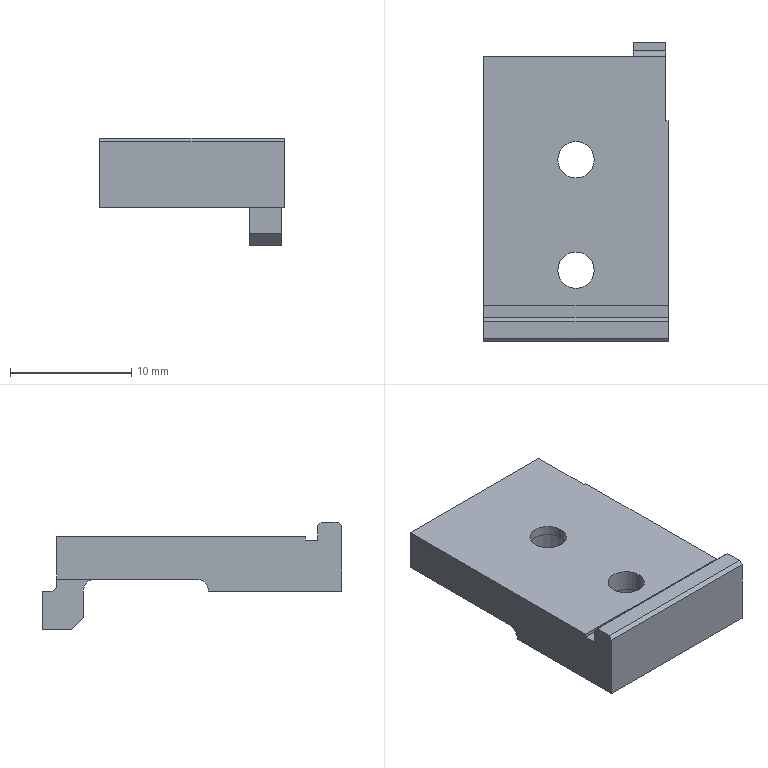Part | NX | 1 solid | 34 faces | box 15.2 x 24.7 x 8.9 mm | volume 1358 mm3 | plane 23 | cylinder 11 | commonest cylinder face diameters 3 x4 5 x4 2 x2 1 x1
STEP:
#1=CARTESIAN_POINT('',(-15.2,-12.7,1.));
#2=VERTEX_POINT('',#1);
#3=CARTESIAN_POINT('',(-15.2,-1.2,1.));
#4=VERTEX_POINT('',#3);
#5=CARTESIAN_POINT('',(-15.2,0.,1.));
#6=DIRECTION('',(0.,1.,0.));
#7=VECTOR('',#6,1000.);
#8=LINE('',#5,#7);
#9=EDGE_CURVE('',#2,#4,#8,.T.);
#10=ORIENTED_EDGE('',*,*,#9,.F.);
#11=CARTESIAN_POINT('',(-15.2,-13.7,0.));
#12=VERTEX_POINT('',#11);
#13=CARTESIAN_POINT('',(-15.2,-12.7,0.));
#14=DIRECTION('',(1.,0.,0.));
#15=DIRECTION('',(0.,-1.,0.));
#16=AXIS2_PLACEMENT_3D('',#13,#14,#15);
#17=CIRCLE('',#16,1.);
#18=EDGE_CURVE('',#2,#12,#17,.T.);
#19=ORIENTED_EDGE('',*,*,#18,.T.);
#20=CARTESIAN_POINT('',(-15.2,-24.7,0.));
#21=VERTEX_POINT('',#20);
#22=CARTESIAN_POINT('',(-15.2,0.,0.));
#23=DIRECTION('',(0.,1.,0.));
#24=VECTOR('',#23,1000.);
#25=LINE('',#22,#24);
#26=EDGE_CURVE('',#21,#12,#25,.T.);
#27=ORIENTED_EDGE('',*,*,#26,.F.);
#28=CARTESIAN_POINT('',(-15.2,-24.7,5.4));
#29=VERTEX_POINT('',#28);
#30=CARTESIAN_POINT('',(-15.2,-24.7,0.));
#31=DIRECTION('',(0.,0.,-1.));
#32=VECTOR('',#31,1000.);
#33=LINE('',#30,#32);
#34=EDGE_CURVE('',#29,#21,#33,.T.);
#35=ORIENTED_EDGE('',*,*,#34,.F.);
#36=CARTESIAN_POINT('',(-15.2,-24.4,5.7));
#37=VERTEX_POINT('',#36);
#38=CARTESIAN_POINT('',(-15.2,0.,30.1));
#39=DIRECTION('',(0.,0.7071,0.7071));
#40=VECTOR('',#39,1000.);
#41=LINE('',#38,#40);
#42=EDGE_CURVE('',#29,#37,#41,.T.);
#43=ORIENTED_EDGE('',*,*,#42,.T.);
#44=CARTESIAN_POINT('',(-15.2,-23.,5.7));
#45=VERTEX_POINT('',#44);
#46=CARTESIAN_POINT('',(-15.2,0.,5.7));
#47=DIRECTION('',(0.,1.,0.));
#48=VECTOR('',#47,1000.);
#49=LINE('',#46,#48);
#50=EDGE_CURVE('',#37,#45,#49,.T.);
#51=ORIENTED_EDGE('',*,*,#50,.T.);
#52=CARTESIAN_POINT('',(-15.2,-22.7,5.4));
#53=VERTEX_POINT('',#52);
#54=CARTESIAN_POINT('',(-15.2,0.,-17.3));
#55=DIRECTION('',(0.,-0.7071,0.7071));
#56=VECTOR('',#55,1000.);
#57=LINE('',#54,#56);
#58=EDGE_CURVE('',#53,#45,#57,.T.);
#59=ORIENTED_EDGE('',*,*,#58,.F.);
#60=CARTESIAN_POINT('',(-15.2,-22.7,4.2));
#61=VERTEX_POINT('',#60);
#62=CARTESIAN_POINT('',(-15.2,-22.7,0.));
#63=DIRECTION('',(0.,0.,-1.));
#64=VECTOR('',#63,1000.);
#65=LINE('',#62,#64);
#66=EDGE_CURVE('',#53,#61,#65,.T.);
#67=ORIENTED_EDGE('',*,*,#66,.T.);
#68=CARTESIAN_POINT('',(-15.2,-21.7,4.2));
#69=VERTEX_POINT('',#68);
#70=CARTESIAN_POINT('',(-15.2,0.,4.2));
#71=DIRECTION('',(0.,-1.,0.));
#72=VECTOR('',#71,1000.);
#73=LINE('',#70,#72);
#74=EDGE_CURVE('',#69,#61,#73,.T.);
#75=ORIENTED_EDGE('',*,*,#74,.F.);
#76=CARTESIAN_POINT('',(-15.2,-21.7,4.5));
#77=VERTEX_POINT('',#76);
#78=CARTESIAN_POINT('',(-15.2,-21.7,0.));
#79=DIRECTION('',(0.,0.,-1.));
#80=VECTOR('',#79,1000.);
#81=LINE('',#78,#80);
#82=EDGE_CURVE('',#77,#69,#81,.T.);
#83=ORIENTED_EDGE('',*,*,#82,.F.);
#84=CARTESIAN_POINT('',(-15.2,-1.2,4.5));
#85=VERTEX_POINT('',#84);
#86=CARTESIAN_POINT('',(-15.2,0.,4.5));
#87=DIRECTION('',(0.,-1.,0.));
#88=VECTOR('',#87,1000.);
#89=LINE('',#86,#88);
#90=EDGE_CURVE('',#85,#77,#89,.T.);
#91=ORIENTED_EDGE('',*,*,#90,.F.);
#92=CARTESIAN_POINT('',(-15.2,-1.2,0.));
#93=DIRECTION('',(0.,0.,1.));
#94=VECTOR('',#93,1000.);
#95=LINE('',#92,#94);
#96=EDGE_CURVE('',#4,#85,#95,.T.);
#97=ORIENTED_EDGE('',*,*,#96,.F.);
#98=EDGE_LOOP('',(#10,#19,#27,#35,#43,#51,#59,#67,#75,#83,#91,#97));
#99=FACE_BOUND('',#98,.T.);
#100=CARTESIAN_POINT('',(-15.2,0.,0.));
#101=DIRECTION('',(1.,0.,0.));
#102=DIRECTION('',(0.,1.,0.));
#103=AXIS2_PLACEMENT_3D('',#100,#101,#102);
#104=PLANE('',#103);
#105=ADVANCED_FACE('',(#99),#104,.F.);
#106=CARTESIAN_POINT('',(0.,-21.7,4.5));
#107=VERTEX_POINT('',#106);
#108=CARTESIAN_POINT('',(0.,-6.5,4.5));
#109=VERTEX_POINT('',#108);
#110=CARTESIAN_POINT('',(0.,0.,4.5));
#111=DIRECTION('',(0.,1.,0.));
#112=VECTOR('',#111,1000.);
#113=LINE('',#110,#112);
#114=EDGE_CURVE('',#107,#109,#113,.T.);
#115=ORIENTED_EDGE('',*,*,#114,.F.);
#116=CARTESIAN_POINT('',(0.,-21.7,4.2));
#117=VERTEX_POINT('',#116);
#118=CARTESIAN_POINT('',(0.,-21.7,0.));
#119=DIRECTION('',(0.,0.,1.));
#120=VECTOR('',#119,1000.);
#121=LINE('',#118,#120);
#122=EDGE_CURVE('',#117,#107,#121,.T.);
#123=ORIENTED_EDGE('',*,*,#122,.F.);
#124=CARTESIAN_POINT('',(0.,-22.7,4.2));
#125=VERTEX_POINT('',#124);
#126=CARTESIAN_POINT('',(0.,0.,4.2));
#127=DIRECTION('',(0.,1.,0.));
#128=VECTOR('',#127,1000.);
#129=LINE('',#126,#128);
#130=EDGE_CURVE('',#125,#117,#129,.T.);
#131=ORIENTED_EDGE('',*,*,#130,.F.);
#132=CARTESIAN_POINT('',(0.,-22.7,5.4));
#133=VERTEX_POINT('',#132);
#134=CARTESIAN_POINT('',(0.,-22.7,0.));
#135=DIRECTION('',(0.,0.,1.));
#136=VECTOR('',#135,1000.);
#137=LINE('',#134,#136);
#138=EDGE_CURVE('',#125,#133,#137,.T.);
#139=ORIENTED_EDGE('',*,*,#138,.T.);
#140=CARTESIAN_POINT('',(0.,-23.,5.7));
#141=VERTEX_POINT('',#140);
#142=CARTESIAN_POINT('',(0.,0.,-17.3));
#143=DIRECTION('',(0.,0.7071,-0.7071));
#144=VECTOR('',#143,1000.);
#145=LINE('',#142,#144);
#146=EDGE_CURVE('',#141,#133,#145,.T.);
#147=ORIENTED_EDGE('',*,*,#146,.F.);
#148=CARTESIAN_POINT('',(0.,-24.4,5.7));
#149=VERTEX_POINT('',#148);
#150=CARTESIAN_POINT('',(0.,0.,5.7));
#151=DIRECTION('',(0.,-1.,0.));
#152=VECTOR('',#151,1000.);
#153=LINE('',#150,#152);
#154=EDGE_CURVE('',#141,#149,#153,.T.);
#155=ORIENTED_EDGE('',*,*,#154,.T.);
#156=CARTESIAN_POINT('',(0.,-24.7,5.4));
#157=VERTEX_POINT('',#156);
#158=CARTESIAN_POINT('',(0.,0.,30.1));
#159=DIRECTION('',(0.,-0.7071,-0.7071));
#160=VECTOR('',#159,1000.);
#161=LINE('',#158,#160);
#162=EDGE_CURVE('',#149,#157,#161,.T.);
#163=ORIENTED_EDGE('',*,*,#162,.T.);
#164=CARTESIAN_POINT('',(0.,-24.7,0.));
#165=VERTEX_POINT('',#164);
#166=CARTESIAN_POINT('',(0.,-24.7,0.));
#167=DIRECTION('',(0.,0.,1.));
#168=VECTOR('',#167,1000.);
#169=LINE('',#166,#168);
#170=EDGE_CURVE('',#165,#157,#169,.T.);
#171=ORIENTED_EDGE('',*,*,#170,.F.);
#172=CARTESIAN_POINT('',(0.,-13.7,0.));
#173=VERTEX_POINT('',#172);
#174=CARTESIAN_POINT('',(0.,0.,0.));
#175=DIRECTION('',(0.,-1.,0.));
#176=VECTOR('',#175,1000.);
#177=LINE('',#174,#176);
#178=EDGE_CURVE('',#173,#165,#177,.T.);
#179=ORIENTED_EDGE('',*,*,#178,.F.);
#180=CARTESIAN_POINT('',(0.,-12.7,1.));
#181=VERTEX_POINT('',#180);
#182=CARTESIAN_POINT('',(0.,-12.7,0.));
#183=DIRECTION('',(1.,0.,0.));
#184=DIRECTION('',(0.,-1.,0.));
#185=AXIS2_PLACEMENT_3D('',#182,#183,#184);
#186=CIRCLE('',#185,1.);
#187=EDGE_CURVE('',#181,#173,#186,.T.);
#188=ORIENTED_EDGE('',*,*,#187,.F.);
#189=CARTESIAN_POINT('',(0.,-6.5,1.));
#190=VERTEX_POINT('',#189);
#191=CARTESIAN_POINT('',(0.,0.,1.));
#192=DIRECTION('',(0.,-1.,0.));
#193=VECTOR('',#192,1000.);
#194=LINE('',#191,#193);
#195=EDGE_CURVE('',#190,#181,#194,.T.);
#196=ORIENTED_EDGE('',*,*,#195,.F.);
#197=CARTESIAN_POINT('',(0.,-6.5,0.));
#198=DIRECTION('',(0.,0.,-1.));
#199=VECTOR('',#198,1000.);
#200=LINE('',#197,#199);
#201=EDGE_CURVE('',#109,#190,#200,.T.);
#202=ORIENTED_EDGE('',*,*,#201,.F.);
#203=EDGE_LOOP('',(#115,#123,#131,#139,#147,#155,#163,#171,#179,#188,#196,#202));
#204=FACE_BOUND('',#203,.T.);
#205=CARTESIAN_POINT('',(0.,-24.7,0.));
#206=DIRECTION('',(-1.,0.,0.));
#207=DIRECTION('',(0.,0.,1.));
#208=AXIS2_PLACEMENT_3D('',#205,#206,#207);
#209=PLANE('',#208);
#210=ADVANCED_FACE('',(#204),#209,.F.);
#211=CARTESIAN_POINT('',(-5.1,-18.8,2.7));
#212=VERTEX_POINT('',#211);
#213=CARTESIAN_POINT('',(-10.1,-18.8,2.7));
#214=VERTEX_POINT('',#213);
#215=CARTESIAN_POINT('',(-7.6,-18.8,2.7));
#216=DIRECTION('',(0.,0.,-1.));
#217=DIRECTION('',(-1.,0.,0.));
#218=AXIS2_PLACEMENT_3D('',#215,#216,#217);
#219=CIRCLE('',#218,2.5);
#220=EDGE_CURVE('',#212,#214,#219,.T.);
#221=ORIENTED_EDGE('',*,*,#220,.T.);
#222=CARTESIAN_POINT('',(-7.6,-18.8,2.7));
#223=DIRECTION('',(0.,0.,-1.));
#224=DIRECTION('',(-1.,0.,0.));
#225=AXIS2_PLACEMENT_3D('',#222,#223,#224);
#226=CIRCLE('',#225,2.5);
#227=EDGE_CURVE('',#214,#212,#226,.T.);
#228=ORIENTED_EDGE('',*,*,#227,.T.);
#229=EDGE_LOOP('',(#221,#228));
#230=FACE_BOUND('',#229,.T.);
#231=CARTESIAN_POINT('',(-6.1,-18.8,2.7));
#232=VERTEX_POINT('',#231);
#233=CARTESIAN_POINT('',(-9.1,-18.8,2.7));
#234=VERTEX_POINT('',#233);
#235=CARTESIAN_POINT('',(-7.6,-18.8,2.7));
#236=DIRECTION('',(0.,0.,-1.));
#237=DIRECTION('',(-1.,0.,0.));
#238=AXIS2_PLACEMENT_3D('',#235,#236,#237);
#239=CIRCLE('',#238,1.5);
#240=EDGE_CURVE('',#232,#234,#239,.T.);
#241=ORIENTED_EDGE('',*,*,#240,.F.);
#242=CARTESIAN_POINT('',(-7.6,-18.8,2.7));
#243=DIRECTION('',(0.,0.,-1.));
#244=DIRECTION('',(-1.,0.,0.));
#245=AXIS2_PLACEMENT_3D('',#242,#243,#244);
#246=CIRCLE('',#245,1.5);
#247=EDGE_CURVE('',#234,#232,#246,.T.);
#248=ORIENTED_EDGE('',*,*,#247,.F.);
#249=EDGE_LOOP('',(#241,#248));
#250=FACE_BOUND('',#249,.T.);
#251=CARTESIAN_POINT('',(-11.486,-5.592,2.7));
#252=DIRECTION('',(0.,0.,-1.));
#253=DIRECTION('',(0.,-1.,0.));
#254=AXIS2_PLACEMENT_3D('',#251,#252,#253);
#255=PLANE('',#254);
#256=ADVANCED_FACE('',(#230,#250),#255,.T.);
#257=CARTESIAN_POINT('',(-0.2,-4.4,1.));
#258=VERTEX_POINT('',#257);
#259=CARTESIAN_POINT('',(-2.9,-4.4,1.));
#260=VERTEX_POINT('',#259);
#261=CARTESIAN_POINT('',(0.,-4.4,1.));
#262=DIRECTION('',(-1.,0.,0.));
#263=VECTOR('',#262,1000.);
#264=LINE('',#261,#263);
#265=EDGE_CURVE('',#258,#260,#264,.T.);
#266=ORIENTED_EDGE('',*,*,#265,.F.);
#267=CARTESIAN_POINT('',(-0.2,-6.5,1.));
#268=VERTEX_POINT('',#267);
#269=CARTESIAN_POINT('',(-0.2,0.,1.));
#270=DIRECTION('',(0.,1.,0.));
#271=VECTOR('',#270,1000.);
#272=LINE('',#269,#271);
#273=EDGE_CURVE('',#268,#258,#272,.T.);
#274=ORIENTED_EDGE('',*,*,#273,.F.);
#275=CARTESIAN_POINT('',(0.,-6.5,1.));
#276=DIRECTION('',(-1.,0.,0.));
#277=VECTOR('',#276,1000.);
#278=LINE('',#275,#277);
#279=EDGE_CURVE('',#190,#268,#278,.T.);
#280=ORIENTED_EDGE('',*,*,#279,.F.);
#281=ORIENTED_EDGE('',*,*,#195,.T.);
#282=CARTESIAN_POINT('',(0.,-12.7,1.));
#283=DIRECTION('',(1.,0.,0.));
#284=VECTOR('',#283,1000.);
#285=LINE('',#282,#284);
#286=EDGE_CURVE('',#2,#181,#285,.T.);
#287=ORIENTED_EDGE('',*,*,#286,.F.);
#288=ORIENTED_EDGE('',*,*,#9,.T.);
#289=CARTESIAN_POINT('',(-2.9,-1.2,1.));
#290=VERTEX_POINT('',#289);
#291=CARTESIAN_POINT('',(0.,-1.2,1.));
#292=DIRECTION('',(-1.,0.,0.));
#293=VECTOR('',#292,1000.);
#294=LINE('',#291,#293);
#295=EDGE_CURVE('',#290,#4,#294,.T.);
#296=ORIENTED_EDGE('',*,*,#295,.F.);
#297=CARTESIAN_POINT('',(-2.9,0.,1.));
#298=DIRECTION('',(0.,1.,0.));
#299=VECTOR('',#298,1000.);
#300=LINE('',#297,#299);
#301=EDGE_CURVE('',#260,#290,#300,.T.);
#302=ORIENTED_EDGE('',*,*,#301,.F.);
#303=EDGE_LOOP('',(#266,#274,#280,#281,#287,#288,#296,#302));
#304=FACE_BOUND('',#303,.T.);
#305=CARTESIAN_POINT('',(-10.1,-9.7,1.));
#306=VERTEX_POINT('',#305);
#307=CARTESIAN_POINT('',(-5.1,-9.7,1.));
#308=VERTEX_POINT('',#307);
#309=CARTESIAN_POINT('',(-7.6,-9.7,1.));
#310=DIRECTION('',(0.,0.,-1.));
#311=DIRECTION('',(-1.,0.,0.));
#312=AXIS2_PLACEMENT_3D('',#309,#310,#311);
#313=CIRCLE('',#312,2.5);
#314=EDGE_CURVE('',#306,#308,#313,.T.);
#315=ORIENTED_EDGE('',*,*,#314,.F.);
#316=CARTESIAN_POINT('',(-7.6,-9.7,1.));
#317=DIRECTION('',(0.,0.,-1.));
#318=DIRECTION('',(-1.,0.,0.));
#319=AXIS2_PLACEMENT_3D('',#316,#317,#318);
#320=CIRCLE('',#319,2.5);
#321=EDGE_CURVE('',#308,#306,#320,.T.);
#322=ORIENTED_EDGE('',*,*,#321,.F.);
#323=EDGE_LOOP('',(#315,#322));
#324=FACE_BOUND('',#323,.T.);
#325=CARTESIAN_POINT('',(-11.724,-4.43,1.));
#326=DIRECTION('',(0.,0.,-1.));
#327=DIRECTION('',(0.,-1.,0.));
#328=AXIS2_PLACEMENT_3D('',#325,#326,#327);
#329=PLANE('',#328);
#330=ADVANCED_FACE('',(#304,#324),#329,.T.);
#331=CARTESIAN_POINT('',(-0.2,-3.4,-2.2));
#332=VERTEX_POINT('',#331);
#333=CARTESIAN_POINT('',(-0.2,-3.4,0.));
#334=VERTEX_POINT('',#333);
#335=CARTESIAN_POINT('',(-0.2,-3.4,0.));
#336=DIRECTION('',(0.,0.,1.));
#337=VECTOR('',#336,1000.);
#338=LINE('',#335,#337);
#339=EDGE_CURVE('',#332,#334,#338,.T.);
#340=ORIENTED_EDGE('',*,*,#339,.F.);
#341=CARTESIAN_POINT('',(-0.2,-2.4,-3.2));
#342=VERTEX_POINT('',#341);
#343=CARTESIAN_POINT('',(-0.2,-5.6,0.));
#344=DIRECTION('',(0.,0.7071,-0.7071));
#345=VECTOR('',#344,1000.);
#346=LINE('',#343,#345);
#347=EDGE_CURVE('',#332,#342,#346,.T.);
#348=ORIENTED_EDGE('',*,*,#347,.T.);
#349=CARTESIAN_POINT('',(-0.2,0.,-3.2));
#350=VERTEX_POINT('',#349);
#351=CARTESIAN_POINT('',(-0.2,0.,-3.2));
#352=DIRECTION('',(0.,-1.,0.));
#353=VECTOR('',#352,1000.);
#354=LINE('',#351,#353);
#355=EDGE_CURVE('',#350,#342,#354,.T.);
#356=ORIENTED_EDGE('',*,*,#355,.F.);
#357=CARTESIAN_POINT('',(-0.2,0.,0.));
#358=VERTEX_POINT('',#357);
#359=CARTESIAN_POINT('',(-0.2,0.,0.));
#360=DIRECTION('',(0.,0.,-1.));
#361=VECTOR('',#360,1000.);
#362=LINE('',#359,#361);
#363=EDGE_CURVE('',#358,#350,#362,.T.);
#364=ORIENTED_EDGE('',*,*,#363,.F.);
#365=CARTESIAN_POINT('',(-0.2,-0.7,0.));
#366=VERTEX_POINT('',#365);
#367=CARTESIAN_POINT('',(-0.2,0.,0.));
#368=DIRECTION('',(0.,-1.,0.));
#369=VECTOR('',#368,1000.);
#370=LINE('',#367,#369);
#371=EDGE_CURVE('',#358,#366,#370,.T.);
#372=ORIENTED_EDGE('',*,*,#371,.T.);
#373=CARTESIAN_POINT('',(-0.2,-1.2,0.5));
#374=VERTEX_POINT('',#373);
#375=CARTESIAN_POINT('',(-0.2,-0.7,0.5));
#376=DIRECTION('',(-1.,0.,0.));
#377=DIRECTION('',(0.,1.,0.));
#378=AXIS2_PLACEMENT_3D('',#375,#376,#377);
#379=CIRCLE('',#378,0.5);
#380=EDGE_CURVE('',#366,#374,#379,.T.);
#381=ORIENTED_EDGE('',*,*,#380,.T.);
#382=CARTESIAN_POINT('',(-0.2,-1.2,4.5));
#383=VERTEX_POINT('',#382);
#384=CARTESIAN_POINT('',(-0.2,-1.2,0.));
#385=DIRECTION('',(0.,0.,1.));
#386=VECTOR('',#385,1000.);
#387=LINE('',#384,#386);
#388=EDGE_CURVE('',#374,#383,#387,.T.);
#389=ORIENTED_EDGE('',*,*,#388,.T.);
#390=CARTESIAN_POINT('',(-0.2,-6.5,4.5));
#391=VERTEX_POINT('',#390);
#392=CARTESIAN_POINT('',(-0.2,0.,4.5));
#393=DIRECTION('',(0.,-1.,0.));
#394=VECTOR('',#393,1000.);
#395=LINE('',#392,#394);
#396=EDGE_CURVE('',#383,#391,#395,.T.);
#397=ORIENTED_EDGE('',*,*,#396,.T.);
#398=CARTESIAN_POINT('',(-0.2,-6.5,0.));
#399=DIRECTION('',(0.,0.,1.));
#400=VECTOR('',#399,1000.);
#401=LINE('',#398,#400);
#402=EDGE_CURVE('',#268,#391,#401,.T.);
#403=ORIENTED_EDGE('',*,*,#402,.F.);
#404=ORIENTED_EDGE('',*,*,#273,.T.);
#405=CARTESIAN_POINT('',(-0.2,-4.4,0.));
#406=DIRECTION('',(-1.,0.,0.));
#407=DIRECTION('',(0.,1.,0.));
#408=AXIS2_PLACEMENT_3D('',#405,#406,#407);
#409=CIRCLE('',#408,1.);
#410=EDGE_CURVE('',#258,#334,#409,.T.);
#411=ORIENTED_EDGE('',*,*,#410,.T.);
#412=EDGE_LOOP('',(#340,#348,#356,#364,#372,#381,#389,#397,#403,#404,#411));
#413=FACE_BOUND('',#412,.T.);
#414=CARTESIAN_POINT('',(-0.2,-6.5,2.));
#415=DIRECTION('',(1.,0.,0.));
#416=DIRECTION('',(0.,1.,0.));
#417=AXIS2_PLACEMENT_3D('',#414,#415,#416);
#418=PLANE('',#417);
#419=ADVANCED_FACE('',(#413),#418,.T.);
#420=ORIENTED_EDGE('',*,*,#82,.T.);
#421=CARTESIAN_POINT('',(0.,-21.7,4.2));
#422=DIRECTION('',(1.,0.,0.));
#423=VECTOR('',#422,1000.);
#424=LINE('',#421,#423);
#425=EDGE_CURVE('',#69,#117,#424,.T.);
#426=ORIENTED_EDGE('',*,*,#425,.T.);
#427=ORIENTED_EDGE('',*,*,#122,.T.);
#428=CARTESIAN_POINT('',(0.,-21.7,4.5));
#429=DIRECTION('',(1.,0.,0.));
#430=VECTOR('',#429,1000.);
#431=LINE('',#428,#430);
#432=EDGE_CURVE('',#77,#107,#431,.T.);
#433=ORIENTED_EDGE('',*,*,#432,.F.);
#434=EDGE_LOOP('',(#420,#426,#427,#433));
#435=FACE_BOUND('',#434,.T.);
#436=CARTESIAN_POINT('',(0.,-21.7,2.));
#437=DIRECTION('',(0.,-1.,0.));
#438=DIRECTION('',(0.,0.,-1.));
#439=AXIS2_PLACEMENT_3D('',#436,#437,#438);
#440=PLANE('',#439);
#441=ADVANCED_FACE('',(#435),#440,.T.);
#442=CARTESIAN_POINT('',(-2.9,-3.4,-2.2));
#443=VERTEX_POINT('',#442);
#444=CARTESIAN_POINT('',(-2.9,-3.4,0.));
#445=VERTEX_POINT('',#444);
#446=CARTESIAN_POINT('',(-2.9,-3.4,0.));
#447=DIRECTION('',(0.,0.,1.));
#448=VECTOR('',#447,1000.);
#449=LINE('',#446,#448);
#450=EDGE_CURVE('',#443,#445,#449,.T.);
#451=ORIENTED_EDGE('',*,*,#450,.T.);
#452=CARTESIAN_POINT('',(-2.9,-4.4,0.));
#453=DIRECTION('',(-1.,0.,0.));
#454=DIRECTION('',(0.,1.,0.));
#455=AXIS2_PLACEMENT_3D('',#452,#453,#454);
#456=CIRCLE('',#455,1.);
#457=EDGE_CURVE('',#260,#445,#456,.T.);
#458=ORIENTED_EDGE('',*,*,#457,.F.);
#459=ORIENTED_EDGE('',*,*,#301,.T.);
#460=CARTESIAN_POINT('',(-2.9,-1.2,0.5));
#461=VERTEX_POINT('',#460);
#462=CARTESIAN_POINT('',(-2.9,-1.2,0.));
#463=DIRECTION('',(0.,0.,1.));
#464=VECTOR('',#463,1000.);
#465=LINE('',#462,#464);
#466=EDGE_CURVE('',#461,#290,#465,.T.);
#467=ORIENTED_EDGE('',*,*,#466,.F.);
#468=CARTESIAN_POINT('',(-2.9,-0.7,0.));
#469=VERTEX_POINT('',#468);
#470=CARTESIAN_POINT('',(-2.9,-0.7,0.5));
#471=DIRECTION('',(-1.,0.,0.));
#472=DIRECTION('',(0.,1.,0.));
#473=AXIS2_PLACEMENT_3D('',#470,#471,#472);
#474=CIRCLE('',#473,0.5);
#475=EDGE_CURVE('',#469,#461,#474,.T.);
#476=ORIENTED_EDGE('',*,*,#475,.F.);
#477=CARTESIAN_POINT('',(-2.9,0.,0.));
#478=VERTEX_POINT('',#477);
#479=CARTESIAN_POINT('',(-2.9,0.,0.));
#480=DIRECTION('',(0.,-1.,0.));
#481=VECTOR('',#480,1000.);
#482=LINE('',#479,#481);
#483=EDGE_CURVE('',#478,#469,#482,.T.);
#484=ORIENTED_EDGE('',*,*,#483,.F.);
#485=CARTESIAN_POINT('',(-2.9,0.,-3.2));
#486=VERTEX_POINT('',#485);
#487=CARTESIAN_POINT('',(-2.9,0.,0.));
#488=DIRECTION('',(0.,0.,-1.));
#489=VECTOR('',#488,1000.);
#490=LINE('',#487,#489);
#491=EDGE_CURVE('',#478,#486,#490,.T.);
#492=ORIENTED_EDGE('',*,*,#491,.T.);
#493=CARTESIAN_POINT('',(-2.9,-2.4,-3.2));
#494=VERTEX_POINT('',#493);
#495=CARTESIAN_POINT('',(-2.9,0.,-3.2));
#496=DIRECTION('',(0.,1.,0.));
#497=VECTOR('',#496,1000.);
#498=LINE('',#495,#497);
#499=EDGE_CURVE('',#494,#486,#498,.T.);
#500=ORIENTED_EDGE('',*,*,#499,.F.);
#501=CARTESIAN_POINT('',(-2.9,-5.6,0.));
#502=DIRECTION('',(0.,0.7071,-0.7071));
#503=VECTOR('',#502,1000.);
#504=LINE('',#501,#503);
#505=EDGE_CURVE('',#443,#494,#504,.T.);
#506=ORIENTED_EDGE('',*,*,#505,.F.);
#507=EDGE_LOOP('',(#451,#458,#459,#467,#476,#484,#492,#500,#506));
#508=FACE_BOUND('',#507,.T.);
#509=CARTESIAN_POINT('',(-2.9,-1.2,0.));
#510=DIRECTION('',(1.,0.,0.));
#511=DIRECTION('',(0.,1.,0.));
#512=AXIS2_PLACEMENT_3D('',#509,#510,#511);
#513=PLANE('',#512);
#514=ADVANCED_FACE('',(#508),#513,.F.);
#515=ORIENTED_EDGE('',*,*,#279,.T.);
#516=ORIENTED_EDGE('',*,*,#402,.T.);
#517=CARTESIAN_POINT('',(0.,-6.5,4.5));
#518=DIRECTION('',(-1.,0.,0.));
#519=VECTOR('',#518,1000.);
#520=LINE('',#517,#519);
#521=EDGE_CURVE('',#109,#391,#520,.T.);
#522=ORIENTED_EDGE('',*,*,#521,.F.);
#523=ORIENTED_EDGE('',*,*,#201,.T.);
#524=EDGE_LOOP('',(#515,#516,#522,#523));
#525=FACE_BOUND('',#524,.T.);
#526=CARTESIAN_POINT('',(0.,-6.5,2.));
#527=DIRECTION('',(0.,1.,0.));
#528=DIRECTION('',(1.,0.,0.));
#529=AXIS2_PLACEMENT_3D('',#526,#527,#528);
#530=PLANE('',#529);
#531=ADVANCED_FACE('',(#525),#530,.T.);
#532=CARTESIAN_POINT('',(0.,-13.7,0.));
#533=DIRECTION('',(1.,0.,0.));
#534=VECTOR('',#533,1000.);
#535=LINE('',#532,#534);
#536=EDGE_CURVE('',#12,#173,#535,.T.);
#537=ORIENTED_EDGE('',*,*,#536,.T.);
#538=ORIENTED_EDGE('',*,*,#178,.T.);
#539=CARTESIAN_POINT('',(-15.2,-24.7,0.));
#540=DIRECTION('',(1.,0.,0.));
#541=VECTOR('',#540,1000.);
#542=LINE('',#539,#541);
#543=EDGE_CURVE('',#21,#165,#542,.T.);
#544=ORIENTED_EDGE('',*,*,#543,.F.);
#545=ORIENTED_EDGE('',*,*,#26,.T.);
#546=EDGE_LOOP('',(#537,#538,#544,#545));
#547=FACE_BOUND('',#546,.T.);
#548=CARTESIAN_POINT('',(-10.1,-18.8,0.));
#549=VERTEX_POINT('',#548);
#550=CARTESIAN_POINT('',(-5.1,-18.8,0.));
#551=VERTEX_POINT('',#550);
#552=CARTESIAN_POINT('',(-7.6,-18.8,0.));
#553=DIRECTION('',(0.,0.,-1.));
#554=DIRECTION('',(-1.,0.,0.));
#555=AXIS2_PLACEMENT_3D('',#552,#553,#554);
#556=CIRCLE('',#555,2.5);
#557=EDGE_CURVE('',#549,#551,#556,.T.);
#558=ORIENTED_EDGE('',*,*,#557,.F.);
#559=CARTESIAN_POINT('',(-7.6,-18.8,0.));
#560=DIRECTION('',(0.,0.,-1.));
#561=DIRECTION('',(-1.,0.,0.));
#562=AXIS2_PLACEMENT_3D('',#559,#560,#561);
#563=CIRCLE('',#562,2.5);
#564=EDGE_CURVE('',#551,#549,#563,.T.);
#565=ORIENTED_EDGE('',*,*,#564,.F.);
#566=EDGE_LOOP('',(#558,#565));
#567=FACE_BOUND('',#566,.T.);
#568=CARTESIAN_POINT('',(-11.977,-15.053,0.));
#569=DIRECTION('',(0.,0.,-1.));
#570=DIRECTION('',(0.,-1.,0.));
#571=AXIS2_PLACEMENT_3D('',#568,#569,#570);
#572=PLANE('',#571);
#573=ADVANCED_FACE('',(#547,#567),#572,.T.);
#574=ORIENTED_EDGE('',*,*,#371,.F.);
#575=CARTESIAN_POINT('',(0.,0.,0.));
#576=DIRECTION('',(1.,0.,0.));
#577=VECTOR('',#576,1000.);
#578=LINE('',#575,#577);
#579=EDGE_CURVE('',#478,#358,#578,.T.);
#580=ORIENTED_EDGE('',*,*,#579,.F.);
#581=ORIENTED_EDGE('',*,*,#483,.T.);
#582=CARTESIAN_POINT('',(0.,-0.7,0.));
#583=DIRECTION('',(-1.,0.,0.));
#584=VECTOR('',#583,1000.);
#585=LINE('',#582,#584);
#586=EDGE_CURVE('',#366,#469,#585,.T.);
#587=ORIENTED_EDGE('',*,*,#586,.F.);
#588=EDGE_LOOP('',(#574,#580,#581,#587));
#589=FACE_BOUND('',#588,.T.);
#590=CARTESIAN_POINT('',(-15.2,-1.2,0.));
#591=DIRECTION('',(0.,0.,1.));
#592=DIRECTION('',(1.,0.,0.));
#593=AXIS2_PLACEMENT_3D('',#590,#591,#592);
#594=PLANE('',#593);
#595=ADVANCED_FACE('',(#589),#594,.T.);
#596=CARTESIAN_POINT('',(0.,0.,-3.2));
#597=DIRECTION('',(1.,0.,0.));
#598=VECTOR('',#597,1000.);
#599=LINE('',#596,#598);
#600=EDGE_CURVE('',#486,#350,#599,.T.);
#601=ORIENTED_EDGE('',*,*,#600,.F.);
#602=ORIENTED_EDGE('',*,*,#491,.F.);
#603=ORIENTED_EDGE('',*,*,#579,.T.);
#604=ORIENTED_EDGE('',*,*,#363,.T.);
#605=EDGE_LOOP('',(#601,#602,#603,#604));
#606=FACE_BOUND('',#605,.T.);
#607=CARTESIAN_POINT('',(0.,0.,0.));
#608=DIRECTION('',(0.,-1.,0.));
#609=DIRECTION('',(0.,0.,-1.));
#610=AXIS2_PLACEMENT_3D('',#607,#608,#609);
#611=PLANE('',#610);
#612=ADVANCED_FACE('',(#606),#611,.F.);
#613=CARTESIAN_POINT('',(0.,-2.4,-3.2));
#614=DIRECTION('',(1.,0.,0.));
#615=VECTOR('',#614,1000.);
#616=LINE('',#613,#615);
#617=EDGE_CURVE('',#494,#342,#616,.T.);
#618=ORIENTED_EDGE('',*,*,#617,.F.);
#619=ORIENTED_EDGE('',*,*,#499,.T.);
#620=ORIENTED_EDGE('',*,*,#600,.T.);
#621=ORIENTED_EDGE('',*,*,#355,.T.);
#622=EDGE_LOOP('',(#618,#619,#620,#621));
#623=FACE_BOUND('',#622,.T.);
#624=CARTESIAN_POINT('',(0.,0.,-3.2));
#625=DIRECTION('',(0.,0.,1.));
#626=DIRECTION('',(1.,0.,0.));
#627=AXIS2_PLACEMENT_3D('',#624,#625,#626);
#628=PLANE('',#627);
#629=ADVANCED_FACE('',(#623),#628,.F.);
#630=CARTESIAN_POINT('',(0.,-22.7,4.2));
#631=DIRECTION('',(1.,0.,0.));
#632=VECTOR('',#631,1000.);
#633=LINE('',#630,#632);
#634=EDGE_CURVE('',#61,#125,#633,.T.);
#635=ORIENTED_EDGE('',*,*,#634,.T.);
#636=ORIENTED_EDGE('',*,*,#130,.T.);
#637=ORIENTED_EDGE('',*,*,#425,.F.);
#638=ORIENTED_EDGE('',*,*,#74,.T.);
#639=EDGE_LOOP('',(#635,#636,#637,#638));
#640=FACE_BOUND('',#639,.T.);
#641=CARTESIAN_POINT('',(0.,-21.7,4.2));
#642=DIRECTION('',(0.,0.,1.));
#643=DIRECTION('',(1.,0.,0.));
#644=AXIS2_PLACEMENT_3D('',#641,#642,#643);
#645=PLANE('',#644);
#646=ADVANCED_FACE('',(#640),#645,.T.);
#647=ORIENTED_EDGE('',*,*,#450,.F.);
#648=CARTESIAN_POINT('',(0.,-3.4,-2.2));
#649=DIRECTION('',(-1.,0.,0.));
#650=VECTOR('',#649,1000.);
#651=LINE('',#648,#650);
#652=EDGE_CURVE('',#332,#443,#651,.T.);
#653=ORIENTED_EDGE('',*,*,#652,.F.);
#654=ORIENTED_EDGE('',*,*,#339,.T.);
#655=CARTESIAN_POINT('',(0.,-3.4,0.));
#656=DIRECTION('',(-1.,0.,0.));
#657=VECTOR('',#656,1000.);
#658=LINE('',#655,#657);
#659=EDGE_CURVE('',#334,#445,#658,.T.);
#660=ORIENTED_EDGE('',*,*,#659,.T.);
#661=EDGE_LOOP('',(#647,#653,#654,#660));
#662=FACE_BOUND('',#661,.T.);
#663=CARTESIAN_POINT('',(-15.2,-3.4,0.));
#664=DIRECTION('',(0.,1.,0.));
#665=DIRECTION('',(1.,0.,0.));
#666=AXIS2_PLACEMENT_3D('',#663,#664,#665);
#667=PLANE('',#666);
#668=ADVANCED_FACE('',(#662),#667,.F.);
#669=CARTESIAN_POINT('',(0.,-1.2,0.5));
#670=DIRECTION('',(-1.,0.,0.));
#671=VECTOR('',#670,1000.);
#672=LINE('',#669,#671);
#673=EDGE_CURVE('',#374,#461,#672,.T.);
#674=ORIENTED_EDGE('',*,*,#673,.T.);
#675=ORIENTED_EDGE('',*,*,#466,.T.);
#676=ORIENTED_EDGE('',*,*,#295,.T.);
#677=ORIENTED_EDGE('',*,*,#96,.T.);
#678=CARTESIAN_POINT('',(0.,-1.2,4.5));
#679=DIRECTION('',(-1.,0.,0.));
#680=VECTOR('',#679,1000.);
#681=LINE('',#678,#680);
#682=EDGE_CURVE('',#383,#85,#681,.T.);
#683=ORIENTED_EDGE('',*,*,#682,.F.);
#684=ORIENTED_EDGE('',*,*,#388,.F.);
#685=EDGE_LOOP('',(#674,#675,#676,#677,#683,#684));
#686=FACE_BOUND('',#685,.T.);
#687=CARTESIAN_POINT('',(-15.2,-1.2,2.));
#688=DIRECTION('',(0.,1.,0.));
#689=DIRECTION('',(1.,0.,0.));
#690=AXIS2_PLACEMENT_3D('',#687,#688,#689);
#691=PLANE('',#690);
#692=ADVANCED_FACE('',(#686),#691,.T.);
#693=ORIENTED_EDGE('',*,*,#286,.T.);
#694=ORIENTED_EDGE('',*,*,#187,.T.);
#695=ORIENTED_EDGE('',*,*,#536,.F.);
#696=ORIENTED_EDGE('',*,*,#18,.F.);
#697=EDGE_LOOP('',(#693,#694,#695,#696));
#698=FACE_BOUND('',#697,.T.);
#699=CARTESIAN_POINT('',(0.,-12.7,0.));
#700=DIRECTION('',(1.,0.,0.));
#701=DIRECTION('',(0.,-1.,0.));
#702=AXIS2_PLACEMENT_3D('',#699,#700,#701);
#703=CYLINDRICAL_SURFACE('',#702,1.);
#704=ADVANCED_FACE('',(#698),#703,.F.);
#705=CARTESIAN_POINT('',(0.,-23.,5.7));
#706=DIRECTION('',(-1.,0.,0.));
#707=VECTOR('',#706,1000.);
#708=LINE('',#705,#707);
#709=EDGE_CURVE('',#141,#45,#708,.T.);
#710=ORIENTED_EDGE('',*,*,#709,.T.);
#711=ORIENTED_EDGE('',*,*,#50,.F.);
#712=CARTESIAN_POINT('',(0.,-24.4,5.7));
#713=DIRECTION('',(-1.,0.,0.));
#714=VECTOR('',#713,1000.);
#715=LINE('',#712,#714);
#716=EDGE_CURVE('',#149,#37,#715,.T.);
#717=ORIENTED_EDGE('',*,*,#716,.F.);
#718=ORIENTED_EDGE('',*,*,#154,.F.);
#719=EDGE_LOOP('',(#710,#711,#717,#718));
#720=FACE_BOUND('',#719,.T.);
#721=CARTESIAN_POINT('',(0.,-22.7,5.7));
#722=DIRECTION('',(0.,0.,-1.));
#723=DIRECTION('',(0.,-1.,0.));
#724=AXIS2_PLACEMENT_3D('',#721,#722,#723);
#725=PLANE('',#724);
#726=ADVANCED_FACE('',(#720),#725,.F.);
#727=ORIENTED_EDGE('',*,*,#634,.F.);
#728=ORIENTED_EDGE('',*,*,#66,.F.);
#729=CARTESIAN_POINT('',(0.,-22.7,5.4));
#730=DIRECTION('',(1.,0.,0.));
#731=VECTOR('',#730,1000.);
#732=LINE('',#729,#731);
#733=EDGE_CURVE('',#53,#133,#732,.T.);
#734=ORIENTED_EDGE('',*,*,#733,.T.);
#735=ORIENTED_EDGE('',*,*,#138,.F.);
#736=EDGE_LOOP('',(#727,#728,#734,#735));
#737=FACE_BOUND('',#736,.T.);
#738=CARTESIAN_POINT('',(0.,-22.7,2.));
#739=DIRECTION('',(0.,-1.,0.));
#740=DIRECTION('',(0.,0.,-1.));
#741=AXIS2_PLACEMENT_3D('',#738,#739,#740);
#742=PLANE('',#741);
#743=ADVANCED_FACE('',(#737),#742,.F.);
#744=ORIENTED_EDGE('',*,*,#709,.F.);
#745=ORIENTED_EDGE('',*,*,#146,.T.);
#746=ORIENTED_EDGE('',*,*,#733,.F.);
#747=ORIENTED_EDGE('',*,*,#58,.T.);
#748=EDGE_LOOP('',(#744,#745,#746,#747));
#749=FACE_BOUND('',#748,.T.);
#750=CARTESIAN_POINT('',(-7.6,-22.85,5.55));
#751=DIRECTION('',(0.,0.7071,0.7071));
#752=DIRECTION('',(1.,0.,0.));
#753=AXIS2_PLACEMENT_3D('',#750,#751,#752);
#754=PLANE('',#753);
#755=ADVANCED_FACE('',(#749),#754,.T.);
#756=ORIENTED_EDGE('',*,*,#557,.T.);
#757=CARTESIAN_POINT('',(-5.1,-18.8,0.));
#758=DIRECTION('',(0.,0.,-1.));
#759=VECTOR('',#758,1000.);
#760=LINE('',#757,#759);
#761=EDGE_CURVE('',#212,#551,#760,.T.);
#762=ORIENTED_EDGE('',*,*,#761,.F.);
#763=ORIENTED_EDGE('',*,*,#227,.F.);
#764=CARTESIAN_POINT('',(-10.1,-18.8,0.));
#765=DIRECTION('',(0.,0.,-1.));
#766=VECTOR('',#765,1000.);
#767=LINE('',#764,#766);
#768=EDGE_CURVE('',#214,#549,#767,.T.);
#769=ORIENTED_EDGE('',*,*,#768,.T.);
#770=EDGE_LOOP('',(#756,#762,#763,#769));
#771=FACE_BOUND('',#770,.T.);
#772=CARTESIAN_POINT('',(-7.6,-18.8,0.));
#773=DIRECTION('',(0.,0.,-1.));
#774=DIRECTION('',(-1.,0.,0.));
#775=AXIS2_PLACEMENT_3D('',#772,#773,#774);
#776=CYLINDRICAL_SURFACE('',#775,2.5);
#777=ADVANCED_FACE('',(#771),#776,.F.);
#778=ORIENTED_EDGE('',*,*,#314,.T.);
#779=CARTESIAN_POINT('',(-5.1,-9.7,3.7));
#780=VERTEX_POINT('',#779);
#781=CARTESIAN_POINT('',(-5.1,-9.7,0.));
#782=DIRECTION('',(0.,0.,-1.));
#783=VECTOR('',#782,1000.);
#784=LINE('',#781,#783);
#785=EDGE_CURVE('',#780,#308,#784,.T.);
#786=ORIENTED_EDGE('',*,*,#785,.F.);
#787=CARTESIAN_POINT('',(-10.1,-9.7,3.7));
#788=VERTEX_POINT('',#787);
#789=CARTESIAN_POINT('',(-7.6,-9.7,3.7));
#790=DIRECTION('',(0.,0.,-1.));
#791=DIRECTION('',(-1.,0.,0.));
#792=AXIS2_PLACEMENT_3D('',#789,#790,#791);
#793=CIRCLE('',#792,2.5);
#794=EDGE_CURVE('',#788,#780,#793,.T.);
#795=ORIENTED_EDGE('',*,*,#794,.F.);
#796=CARTESIAN_POINT('',(-10.1,-9.7,0.));
#797=DIRECTION('',(0.,0.,-1.));
#798=VECTOR('',#797,1000.);
#799=LINE('',#796,#798);
#800=EDGE_CURVE('',#788,#306,#799,.T.);
#801=ORIENTED_EDGE('',*,*,#800,.T.);
#802=EDGE_LOOP('',(#778,#786,#795,#801));
#803=FACE_BOUND('',#802,.T.);
#804=CARTESIAN_POINT('',(-7.6,-9.7,0.));
#805=DIRECTION('',(0.,0.,-1.));
#806=DIRECTION('',(-1.,0.,0.));
#807=AXIS2_PLACEMENT_3D('',#804,#805,#806);
#808=CYLINDRICAL_SURFACE('',#807,2.5);
#809=ADVANCED_FACE('',(#803),#808,.F.);
#810=CARTESIAN_POINT('',(0.,-24.7,5.4));
#811=DIRECTION('',(1.,0.,0.));
#812=VECTOR('',#811,1000.);
#813=LINE('',#810,#812);
#814=EDGE_CURVE('',#29,#157,#813,.T.);
#815=ORIENTED_EDGE('',*,*,#814,.T.);
#816=ORIENTED_EDGE('',*,*,#162,.F.);
#817=ORIENTED_EDGE('',*,*,#716,.T.);
#818=ORIENTED_EDGE('',*,*,#42,.F.);
#819=EDGE_LOOP('',(#815,#816,#817,#818));
#820=FACE_BOUND('',#819,.T.);
#821=CARTESIAN_POINT('',(-7.6,-24.55,5.55));
#822=DIRECTION('',(0.,0.7071,-0.7071));
#823=DIRECTION('',(-1.,0.,0.));
#824=AXIS2_PLACEMENT_3D('',#821,#822,#823);
#825=PLANE('',#824);
#826=ADVANCED_FACE('',(#820),#825,.F.);
#827=CARTESIAN_POINT('',(-9.1,-9.7,4.5));
#828=VERTEX_POINT('',#827);
#829=CARTESIAN_POINT('',(-6.1,-9.7,4.5));
#830=VERTEX_POINT('',#829);
#831=CARTESIAN_POINT('',(-7.6,-9.7,4.5));
#832=DIRECTION('',(0.,0.,-1.));
#833=DIRECTION('',(-1.,0.,0.));
#834=AXIS2_PLACEMENT_3D('',#831,#832,#833);
#835=CIRCLE('',#834,1.5);
#836=EDGE_CURVE('',#828,#830,#835,.T.);
#837=ORIENTED_EDGE('',*,*,#836,.F.);
#838=CARTESIAN_POINT('',(-9.1,-9.7,3.7));
#839=VERTEX_POINT('',#838);
#840=CARTESIAN_POINT('',(-9.1,-9.7,5.45));
#841=DIRECTION('',(0.,0.,-1.));
#842=VECTOR('',#841,1000.);
#843=LINE('',#840,#842);
#844=EDGE_CURVE('',#839,#828,#843,.F.);
#845=ORIENTED_EDGE('',*,*,#844,.F.);
#846=CARTESIAN_POINT('',(-6.1,-9.7,3.7));
#847=VERTEX_POINT('',#846);
#848=CARTESIAN_POINT('',(-7.6,-9.7,3.7));
#849=DIRECTION('',(0.,0.,-1.));
#850=DIRECTION('',(-1.,0.,0.));
#851=AXIS2_PLACEMENT_3D('',#848,#849,#850);
#852=CIRCLE('',#851,1.5);
#853=EDGE_CURVE('',#839,#847,#852,.T.);
#854=ORIENTED_EDGE('',*,*,#853,.T.);
#855=CARTESIAN_POINT('',(-6.1,-9.7,5.45));
#856=DIRECTION('',(0.,0.,-1.));
#857=VECTOR('',#856,1000.);
#858=LINE('',#855,#857);
#859=EDGE_CURVE('',#847,#830,#858,.F.);
#860=ORIENTED_EDGE('',*,*,#859,.T.);
#861=EDGE_LOOP('',(#837,#845,#854,#860));
#862=FACE_BOUND('',#861,.T.);
#863=CARTESIAN_POINT('',(-7.6,-9.7,5.45));
#864=DIRECTION('',(0.,0.,-1.));
#865=DIRECTION('',(-1.,0.,0.));
#866=AXIS2_PLACEMENT_3D('',#863,#864,#865);
#867=CYLINDRICAL_SURFACE('',#866,1.5);
#868=ADVANCED_FACE('',(#862),#867,.F.);
#869=ORIENTED_EDGE('',*,*,#240,.T.);
#870=CARTESIAN_POINT('',(-9.1,-18.8,4.5));
#871=VERTEX_POINT('',#870);
#872=CARTESIAN_POINT('',(-9.1,-18.8,5.45));
#873=DIRECTION('',(0.,0.,-1.));
#874=VECTOR('',#873,1000.);
#875=LINE('',#872,#874);
#876=EDGE_CURVE('',#234,#871,#875,.F.);
#877=ORIENTED_EDGE('',*,*,#876,.T.);
#878=CARTESIAN_POINT('',(-6.1,-18.8,4.5));
#879=VERTEX_POINT('',#878);
#880=CARTESIAN_POINT('',(-7.6,-18.8,4.5));
#881=DIRECTION('',(0.,0.,-1.));
#882=DIRECTION('',(-1.,0.,0.));
#883=AXIS2_PLACEMENT_3D('',#880,#881,#882);
#884=CIRCLE('',#883,1.5);
#885=EDGE_CURVE('',#879,#871,#884,.T.);
#886=ORIENTED_EDGE('',*,*,#885,.F.);
#887=CARTESIAN_POINT('',(-6.1,-18.8,5.45));
#888=DIRECTION('',(0.,0.,-1.));
#889=VECTOR('',#888,1000.);
#890=LINE('',#887,#889);
#891=EDGE_CURVE('',#232,#879,#890,.F.);
#892=ORIENTED_EDGE('',*,*,#891,.F.);
#893=EDGE_LOOP('',(#869,#877,#886,#892));
#894=FACE_BOUND('',#893,.T.);
#895=CARTESIAN_POINT('',(-7.6,-18.8,5.45));
#896=DIRECTION('',(0.,0.,-1.));
#897=DIRECTION('',(-1.,0.,0.));
#898=AXIS2_PLACEMENT_3D('',#895,#896,#897);
#899=CYLINDRICAL_SURFACE('',#898,1.5);
#900=ADVANCED_FACE('',(#894),#899,.F.);
#901=ORIENTED_EDGE('',*,*,#396,.F.);
#902=ORIENTED_EDGE('',*,*,#682,.T.);
#903=ORIENTED_EDGE('',*,*,#90,.T.);
#904=ORIENTED_EDGE('',*,*,#432,.T.);
#905=ORIENTED_EDGE('',*,*,#114,.T.);
#906=ORIENTED_EDGE('',*,*,#521,.T.);
#907=EDGE_LOOP('',(#901,#902,#903,#904,#905,#906));
#908=FACE_BOUND('',#907,.T.);
#909=ORIENTED_EDGE('',*,*,#836,.T.);
#910=CARTESIAN_POINT('',(-7.6,-9.7,4.5));
#911=DIRECTION('',(0.,0.,-1.));
#912=DIRECTION('',(-1.,0.,0.));
#913=AXIS2_PLACEMENT_3D('',#910,#911,#912);
#914=CIRCLE('',#913,1.5);
#915=EDGE_CURVE('',#830,#828,#914,.T.);
#916=ORIENTED_EDGE('',*,*,#915,.T.);
#917=EDGE_LOOP('',(#909,#916));
#918=FACE_BOUND('',#917,.T.);
#919=CARTESIAN_POINT('',(-7.6,-18.8,4.5));
#920=DIRECTION('',(0.,0.,-1.));
#921=DIRECTION('',(-1.,0.,0.));
#922=AXIS2_PLACEMENT_3D('',#919,#920,#921);
#923=CIRCLE('',#922,1.5);
#924=EDGE_CURVE('',#871,#879,#923,.T.);
#925=ORIENTED_EDGE('',*,*,#924,.T.);
#926=ORIENTED_EDGE('',*,*,#885,.T.);
#927=EDGE_LOOP('',(#925,#926));
#928=FACE_BOUND('',#927,.T.);
#929=CARTESIAN_POINT('',(0.,0.,4.5));
#930=DIRECTION('',(0.,0.,1.));
#931=DIRECTION('',(1.,0.,0.));
#932=AXIS2_PLACEMENT_3D('',#929,#930,#931);
#933=PLANE('',#932);
#934=ADVANCED_FACE('',(#908,#918,#928),#933,.T.);
#935=CARTESIAN_POINT('',(-7.6,-9.7,3.7));
#936=DIRECTION('',(0.,0.,-1.));
#937=DIRECTION('',(-1.,0.,0.));
#938=AXIS2_PLACEMENT_3D('',#935,#936,#937);
#939=CIRCLE('',#938,2.5);
#940=EDGE_CURVE('',#780,#788,#939,.T.);
#941=ORIENTED_EDGE('',*,*,#940,.T.);
#942=ORIENTED_EDGE('',*,*,#794,.T.);
#943=EDGE_LOOP('',(#941,#942));
#944=FACE_BOUND('',#943,.T.);
#945=CARTESIAN_POINT('',(-7.6,-9.7,3.7));
#946=DIRECTION('',(0.,0.,-1.));
#947=DIRECTION('',(-1.,0.,0.));
#948=AXIS2_PLACEMENT_3D('',#945,#946,#947);
#949=CIRCLE('',#948,1.5);
#950=EDGE_CURVE('',#847,#839,#949,.T.);
#951=ORIENTED_EDGE('',*,*,#950,.F.);
#952=ORIENTED_EDGE('',*,*,#853,.F.);
#953=EDGE_LOOP('',(#951,#952));
#954=FACE_BOUND('',#953,.T.);
#955=CARTESIAN_POINT('',(-11.486,-5.592,3.7));
#956=DIRECTION('',(0.,0.,-1.));
#957=DIRECTION('',(0.,-1.,0.));
#958=AXIS2_PLACEMENT_3D('',#955,#956,#957);
#959=PLANE('',#958);
#960=ADVANCED_FACE('',(#944,#954),#959,.T.);
#961=ORIENTED_EDGE('',*,*,#673,.F.);
#962=ORIENTED_EDGE('',*,*,#380,.F.);
#963=ORIENTED_EDGE('',*,*,#586,.T.);
#964=ORIENTED_EDGE('',*,*,#475,.T.);
#965=EDGE_LOOP('',(#961,#962,#963,#964));
#966=FACE_BOUND('',#965,.T.);
#967=CARTESIAN_POINT('',(0.,-0.7,0.5));
#968=DIRECTION('',(-1.,0.,0.));
#969=DIRECTION('',(0.,1.,0.));
#970=AXIS2_PLACEMENT_3D('',#967,#968,#969);
#971=CYLINDRICAL_SURFACE('',#970,0.5);
#972=ADVANCED_FACE('',(#966),#971,.F.);
#973=ORIENTED_EDGE('',*,*,#34,.T.);
#974=ORIENTED_EDGE('',*,*,#543,.T.);
#975=ORIENTED_EDGE('',*,*,#170,.T.);
#976=ORIENTED_EDGE('',*,*,#814,.F.);
#977=EDGE_LOOP('',(#973,#974,#975,#976));
#978=FACE_BOUND('',#977,.T.);
#979=CARTESIAN_POINT('',(-15.2,-24.7,1.));
#980=DIRECTION('',(0.,-1.,0.));
#981=DIRECTION('',(0.,0.,-1.));
#982=AXIS2_PLACEMENT_3D('',#979,#980,#981);
#983=PLANE('',#982);
#984=ADVANCED_FACE('',(#978),#983,.T.);
#985=ORIENTED_EDGE('',*,*,#265,.T.);
#986=ORIENTED_EDGE('',*,*,#457,.T.);
#987=ORIENTED_EDGE('',*,*,#659,.F.);
#988=ORIENTED_EDGE('',*,*,#410,.F.);
#989=EDGE_LOOP('',(#985,#986,#987,#988));
#990=FACE_BOUND('',#989,.T.);
#991=CARTESIAN_POINT('',(0.,-4.4,0.));
#992=DIRECTION('',(-1.,0.,0.));
#993=DIRECTION('',(0.,1.,0.));
#994=AXIS2_PLACEMENT_3D('',#991,#992,#993);
#995=CYLINDRICAL_SURFACE('',#994,1.);
#996=ADVANCED_FACE('',(#990),#995,.F.);
#997=ORIENTED_EDGE('',*,*,#617,.T.);
#998=ORIENTED_EDGE('',*,*,#347,.F.);
#999=ORIENTED_EDGE('',*,*,#652,.T.);
#1000=ORIENTED_EDGE('',*,*,#505,.T.);
#1001=EDGE_LOOP('',(#997,#998,#999,#1000));
#1002=FACE_BOUND('',#1001,.T.);
#1003=CARTESIAN_POINT('',(-1.55,-2.9,-2.7));
#1004=DIRECTION('',(0.,-0.7071,-0.7071));
#1005=DIRECTION('',(0.,-0.7071,0.7071));
#1006=AXIS2_PLACEMENT_3D('',#1003,#1004,#1005);
#1007=PLANE('',#1006);
#1008=ADVANCED_FACE('',(#1002),#1007,.T.);
#1009=ORIENTED_EDGE('',*,*,#950,.T.);
#1010=ORIENTED_EDGE('',*,*,#844,.T.);
#1011=ORIENTED_EDGE('',*,*,#915,.F.);
#1012=ORIENTED_EDGE('',*,*,#859,.F.);
#1013=EDGE_LOOP('',(#1009,#1010,#1011,#1012));
#1014=FACE_BOUND('',#1013,.T.);
#1015=CARTESIAN_POINT('',(-7.6,-9.7,5.45));
#1016=DIRECTION('',(0.,0.,-1.));
#1017=DIRECTION('',(-1.,0.,0.));
#1018=AXIS2_PLACEMENT_3D('',#1015,#1016,#1017);
#1019=CYLINDRICAL_SURFACE('',#1018,1.5);
#1020=ADVANCED_FACE('',(#1014),#1019,.F.);
#1021=ORIENTED_EDGE('',*,*,#924,.F.);
#1022=ORIENTED_EDGE('',*,*,#876,.F.);
#1023=ORIENTED_EDGE('',*,*,#247,.T.);
#1024=ORIENTED_EDGE('',*,*,#891,.T.);
#1025=EDGE_LOOP('',(#1021,#1022,#1023,#1024));
#1026=FACE_BOUND('',#1025,.T.);
#1027=CARTESIAN_POINT('',(-7.6,-18.8,5.45));
#1028=DIRECTION('',(0.,0.,-1.));
#1029=DIRECTION('',(-1.,0.,0.));
#1030=AXIS2_PLACEMENT_3D('',#1027,#1028,#1029);
#1031=CYLINDRICAL_SURFACE('',#1030,1.5);
#1032=ADVANCED_FACE('',(#1026),#1031,.F.);
#1033=ORIENTED_EDGE('',*,*,#220,.F.);
#1034=ORIENTED_EDGE('',*,*,#761,.T.);
#1035=ORIENTED_EDGE('',*,*,#564,.T.);
#1036=ORIENTED_EDGE('',*,*,#768,.F.);
#1037=EDGE_LOOP('',(#1033,#1034,#1035,#1036));
#1038=FACE_BOUND('',#1037,.T.);
#1039=CARTESIAN_POINT('',(-7.6,-18.8,0.));
#1040=DIRECTION('',(0.,0.,-1.));
#1041=DIRECTION('',(-1.,0.,0.));
#1042=AXIS2_PLACEMENT_3D('',#1039,#1040,#1041);
#1043=CYLINDRICAL_SURFACE('',#1042,2.5);
#1044=ADVANCED_FACE('',(#1038),#1043,.F.);
#1045=ORIENTED_EDGE('',*,*,#940,.F.);
#1046=ORIENTED_EDGE('',*,*,#785,.T.);
#1047=ORIENTED_EDGE('',*,*,#321,.T.);
#1048=ORIENTED_EDGE('',*,*,#800,.F.);
#1049=EDGE_LOOP('',(#1045,#1046,#1047,#1048));
#1050=FACE_BOUND('',#1049,.T.);
#1051=CARTESIAN_POINT('',(-7.6,-9.7,0.));
#1052=DIRECTION('',(0.,0.,-1.));
#1053=DIRECTION('',(-1.,0.,0.));
#1054=AXIS2_PLACEMENT_3D('',#1051,#1052,#1053);
#1055=CYLINDRICAL_SURFACE('',#1054,2.5);
#1056=ADVANCED_FACE('',(#1050),#1055,.F.);
#1057=CLOSED_SHELL('',(#105,#210,#256,#330,#419,#441,#514,#531,#573,#595,#612,#629,#646,#668,#692,#704,#726,#743,#755,#777,#809,#826,#868,#900,#934,#960,#972,#984,#996,#1008,#1020,#1032,#1044,#1056));
#1058=MANIFOLD_SOLID_BREP('',#1057);
#1059=(LENGTH_UNIT()NAMED_UNIT(*)SI_UNIT(.MILLI.,.METRE.));
#1060=UNCERTAINTY_MEASURE_WITH_UNIT(LENGTH_MEASURE(0.00001),#1059,'','');
#1061=(NAMED_UNIT(*)PLANE_ANGLE_UNIT()SI_UNIT($,.RADIAN.));
#1062=(NAMED_UNIT(*)SI_UNIT($,.STERADIAN.)SOLID_ANGLE_UNIT());
#1063=(GEOMETRIC_REPRESENTATION_CONTEXT(3)GLOBAL_UNCERTAINTY_ASSIGNED_CONTEXT((#1060))GLOBAL_UNIT_ASSIGNED_CONTEXT((#1059,#1061,#1062))REPRESENTATION_CONTEXT('',''));
#1064=ADVANCED_BREP_SHAPE_REPRESENTATION('',(#1058),#1063);